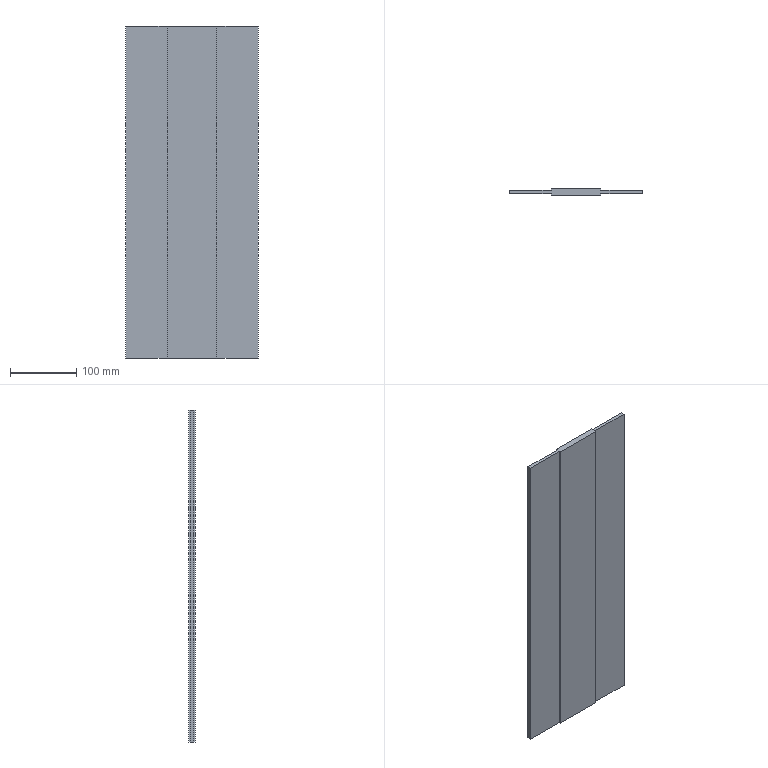Part | SolidWorks | features Extrusion 1, ICE 1 | 1 solid | 14 faces | box 200 x 10 x 500 mm | volume 687500 mm3 | plane 14
STEP:
#1=CARTESIAN_POINT('',(100.,2.5,0.));
#2=VERTEX_POINT('',#1);
#3=CARTESIAN_POINT('',(37.5,2.5,0.));
#4=VERTEX_POINT('',#3);
#5=CARTESIAN_POINT('',(-100.,2.5,0.));
#6=DIRECTION('',(-1.,0.,0.));
#7=VECTOR('',#6,1000.);
#8=LINE('',#5,#7);
#9=EDGE_CURVE('',#2,#4,#8,.T.);
#10=ORIENTED_EDGE('',*,*,#9,.T.);
#11=CARTESIAN_POINT('',(37.5,2.5,500.));
#12=VERTEX_POINT('',#11);
#13=CARTESIAN_POINT('',(37.5,2.5,500.));
#14=DIRECTION('',(0.,0.,1.));
#15=VECTOR('',#14,1000.);
#16=LINE('',#13,#15);
#17=EDGE_CURVE('',#4,#12,#16,.T.);
#18=ORIENTED_EDGE('',*,*,#17,.T.);
#19=CARTESIAN_POINT('',(100.,2.5,500.));
#20=VERTEX_POINT('',#19);
#21=CARTESIAN_POINT('',(-100.,2.5,500.));
#22=DIRECTION('',(-1.,0.,0.));
#23=VECTOR('',#22,1000.);
#24=LINE('',#21,#23);
#25=EDGE_CURVE('',#20,#12,#24,.T.);
#26=ORIENTED_EDGE('',*,*,#25,.F.);
#27=CARTESIAN_POINT('',(100.,2.5,500.));
#28=DIRECTION('',(0.,0.,-1.));
#29=VECTOR('',#28,1000.);
#30=LINE('',#27,#29);
#31=EDGE_CURVE('',#20,#2,#30,.T.);
#32=ORIENTED_EDGE('',*,*,#31,.T.);
#33=EDGE_LOOP('',(#10,#18,#26,#32));
#34=FACE_OUTER_BOUND('',#33,.T.);
#35=CARTESIAN_POINT('',(-100.,2.5,500.));
#36=DIRECTION('',(0.,-1.,0.));
#37=DIRECTION('',(0.,0.,-1.));
#38=AXIS2_PLACEMENT_3D('',#35,#36,#37);
#39=PLANE('',#38);
#40=ADVANCED_FACE('',(#34),#39,.F.);
#41=CARTESIAN_POINT('',(37.5,-2.5,500.));
#42=VERTEX_POINT('',#41);
#43=CARTESIAN_POINT('',(100.,-2.5,500.));
#44=VERTEX_POINT('',#43);
#45=CARTESIAN_POINT('',(-100.,-2.5,500.));
#46=DIRECTION('',(1.,0.,0.));
#47=VECTOR('',#46,1000.);
#48=LINE('',#45,#47);
#49=EDGE_CURVE('',#42,#44,#48,.T.);
#50=ORIENTED_EDGE('',*,*,#49,.F.);
#51=CARTESIAN_POINT('',(37.5,-2.5,0.));
#52=VERTEX_POINT('',#51);
#53=CARTESIAN_POINT('',(37.5,-2.5,500.));
#54=DIRECTION('',(0.,0.,-1.));
#55=VECTOR('',#54,1000.);
#56=LINE('',#53,#55);
#57=EDGE_CURVE('',#42,#52,#56,.T.);
#58=ORIENTED_EDGE('',*,*,#57,.T.);
#59=CARTESIAN_POINT('',(100.,-2.5,0.));
#60=VERTEX_POINT('',#59);
#61=CARTESIAN_POINT('',(-100.,-2.5,0.));
#62=DIRECTION('',(1.,0.,0.));
#63=VECTOR('',#62,1000.);
#64=LINE('',#61,#63);
#65=EDGE_CURVE('',#52,#60,#64,.T.);
#66=ORIENTED_EDGE('',*,*,#65,.T.);
#67=CARTESIAN_POINT('',(100.,-2.5,500.));
#68=DIRECTION('',(0.,0.,-1.));
#69=VECTOR('',#68,1000.);
#70=LINE('',#67,#69);
#71=EDGE_CURVE('',#44,#60,#70,.T.);
#72=ORIENTED_EDGE('',*,*,#71,.F.);
#73=EDGE_LOOP('',(#50,#58,#66,#72));
#74=FACE_OUTER_BOUND('',#73,.T.);
#75=CARTESIAN_POINT('',(-100.,-2.5,500.));
#76=DIRECTION('',(0.,1.,0.));
#77=DIRECTION('',(0.,0.,1.));
#78=AXIS2_PLACEMENT_3D('',#75,#76,#77);
#79=PLANE('',#78);
#80=ADVANCED_FACE('',(#74),#79,.F.);
#81=CARTESIAN_POINT('',(100.,2.5,0.));
#82=DIRECTION('',(0.,1.,0.));
#83=VECTOR('',#82,1000.);
#84=LINE('',#81,#83);
#85=EDGE_CURVE('',#60,#2,#84,.T.);
#86=ORIENTED_EDGE('',*,*,#85,.T.);
#87=ORIENTED_EDGE('',*,*,#31,.F.);
#88=CARTESIAN_POINT('',(100.,2.5,500.));
#89=DIRECTION('',(0.,1.,0.));
#90=VECTOR('',#89,1000.);
#91=LINE('',#88,#90);
#92=EDGE_CURVE('',#44,#20,#91,.T.);
#93=ORIENTED_EDGE('',*,*,#92,.F.);
#94=ORIENTED_EDGE('',*,*,#71,.T.);
#95=EDGE_LOOP('',(#86,#87,#93,#94));
#96=FACE_OUTER_BOUND('',#95,.T.);
#97=CARTESIAN_POINT('',(100.,2.5,500.));
#98=DIRECTION('',(-1.,0.,0.));
#99=DIRECTION('',(0.,0.,1.));
#100=AXIS2_PLACEMENT_3D('',#97,#98,#99);
#101=PLANE('',#100);
#102=ADVANCED_FACE('',(#96),#101,.F.);
#103=CARTESIAN_POINT('',(-37.5,2.5,500.));
#104=VERTEX_POINT('',#103);
#105=CARTESIAN_POINT('',(-100.,2.5,500.));
#106=VERTEX_POINT('',#105);
#107=CARTESIAN_POINT('',(-100.,2.5,500.));
#108=DIRECTION('',(-1.,0.,0.));
#109=VECTOR('',#108,1000.);
#110=LINE('',#107,#109);
#111=EDGE_CURVE('',#104,#106,#110,.T.);
#112=ORIENTED_EDGE('',*,*,#111,.F.);
#113=CARTESIAN_POINT('',(-37.5,2.5,0.));
#114=VERTEX_POINT('',#113);
#115=CARTESIAN_POINT('',(-37.5,2.5,500.));
#116=DIRECTION('',(0.,0.,-1.));
#117=VECTOR('',#116,1000.);
#118=LINE('',#115,#117);
#119=EDGE_CURVE('',#104,#114,#118,.T.);
#120=ORIENTED_EDGE('',*,*,#119,.T.);
#121=CARTESIAN_POINT('',(-100.,2.5,0.));
#122=VERTEX_POINT('',#121);
#123=CARTESIAN_POINT('',(-100.,2.5,0.));
#124=DIRECTION('',(-1.,0.,0.));
#125=VECTOR('',#124,1000.);
#126=LINE('',#123,#125);
#127=EDGE_CURVE('',#114,#122,#126,.T.);
#128=ORIENTED_EDGE('',*,*,#127,.T.);
#129=CARTESIAN_POINT('',(-100.,2.5,500.));
#130=DIRECTION('',(0.,0.,-1.));
#131=VECTOR('',#130,1000.);
#132=LINE('',#129,#131);
#133=EDGE_CURVE('',#106,#122,#132,.T.);
#134=ORIENTED_EDGE('',*,*,#133,.F.);
#135=EDGE_LOOP('',(#112,#120,#128,#134));
#136=FACE_OUTER_BOUND('',#135,.T.);
#137=CARTESIAN_POINT('',(-100.,2.5,500.));
#138=DIRECTION('',(0.,-1.,0.));
#139=DIRECTION('',(0.,0.,-1.));
#140=AXIS2_PLACEMENT_3D('',#137,#138,#139);
#141=PLANE('',#140);
#142=ADVANCED_FACE('',(#136),#141,.F.);
#143=CARTESIAN_POINT('',(-100.,-2.5,0.));
#144=VERTEX_POINT('',#143);
#145=CARTESIAN_POINT('',(-100.,2.5,0.));
#146=DIRECTION('',(0.,-1.,0.));
#147=VECTOR('',#146,1000.);
#148=LINE('',#145,#147);
#149=EDGE_CURVE('',#122,#144,#148,.T.);
#150=ORIENTED_EDGE('',*,*,#149,.T.);
#151=CARTESIAN_POINT('',(-100.,-2.5,500.));
#152=VERTEX_POINT('',#151);
#153=CARTESIAN_POINT('',(-100.,-2.5,500.));
#154=DIRECTION('',(0.,0.,-1.));
#155=VECTOR('',#154,1000.);
#156=LINE('',#153,#155);
#157=EDGE_CURVE('',#152,#144,#156,.T.);
#158=ORIENTED_EDGE('',*,*,#157,.F.);
#159=CARTESIAN_POINT('',(-100.,2.5,500.));
#160=DIRECTION('',(0.,-1.,0.));
#161=VECTOR('',#160,1000.);
#162=LINE('',#159,#161);
#163=EDGE_CURVE('',#106,#152,#162,.T.);
#164=ORIENTED_EDGE('',*,*,#163,.F.);
#165=ORIENTED_EDGE('',*,*,#133,.T.);
#166=EDGE_LOOP('',(#150,#158,#164,#165));
#167=FACE_OUTER_BOUND('',#166,.T.);
#168=CARTESIAN_POINT('',(-100.,2.5,500.));
#169=DIRECTION('',(1.,0.,0.));
#170=DIRECTION('',(0.,0.,-1.));
#171=AXIS2_PLACEMENT_3D('',#168,#169,#170);
#172=PLANE('',#171);
#173=ADVANCED_FACE('',(#167),#172,.F.);
#174=CARTESIAN_POINT('',(-37.5,-2.5,0.));
#175=VERTEX_POINT('',#174);
#176=CARTESIAN_POINT('',(-100.,-2.5,0.));
#177=DIRECTION('',(1.,0.,0.));
#178=VECTOR('',#177,1000.);
#179=LINE('',#176,#178);
#180=EDGE_CURVE('',#144,#175,#179,.T.);
#181=ORIENTED_EDGE('',*,*,#180,.T.);
#182=CARTESIAN_POINT('',(-37.5,-2.5,500.));
#183=VERTEX_POINT('',#182);
#184=CARTESIAN_POINT('',(-37.5,-2.5,500.));
#185=DIRECTION('',(0.,0.,1.));
#186=VECTOR('',#185,1000.);
#187=LINE('',#184,#186);
#188=EDGE_CURVE('',#175,#183,#187,.T.);
#189=ORIENTED_EDGE('',*,*,#188,.T.);
#190=CARTESIAN_POINT('',(-100.,-2.5,500.));
#191=DIRECTION('',(1.,0.,0.));
#192=VECTOR('',#191,1000.);
#193=LINE('',#190,#192);
#194=EDGE_CURVE('',#152,#183,#193,.T.);
#195=ORIENTED_EDGE('',*,*,#194,.F.);
#196=ORIENTED_EDGE('',*,*,#157,.T.);
#197=EDGE_LOOP('',(#181,#189,#195,#196));
#198=FACE_OUTER_BOUND('',#197,.T.);
#199=CARTESIAN_POINT('',(-100.,-2.5,500.));
#200=DIRECTION('',(0.,1.,0.));
#201=DIRECTION('',(0.,0.,1.));
#202=AXIS2_PLACEMENT_3D('',#199,#200,#201);
#203=PLANE('',#202);
#204=ADVANCED_FACE('',(#198),#203,.F.);
#205=ORIENTED_EDGE('',*,*,#194,.T.);
#206=CARTESIAN_POINT('',(-37.5,-5.,500.));
#207=VERTEX_POINT('',#206);
#208=CARTESIAN_POINT('',(-37.5,5.,500.));
#209=DIRECTION('',(0.,-1.,0.));
#210=VECTOR('',#209,1000.);
#211=LINE('',#208,#210);
#212=EDGE_CURVE('',#183,#207,#211,.T.);
#213=ORIENTED_EDGE('',*,*,#212,.T.);
#214=CARTESIAN_POINT('',(37.5,-5.,500.));
#215=VERTEX_POINT('',#214);
#216=CARTESIAN_POINT('',(-37.5,-5.,500.));
#217=DIRECTION('',(1.,0.,0.));
#218=VECTOR('',#217,1000.);
#219=LINE('',#216,#218);
#220=EDGE_CURVE('',#207,#215,#219,.T.);
#221=ORIENTED_EDGE('',*,*,#220,.T.);
#222=CARTESIAN_POINT('',(37.5,5.,500.));
#223=DIRECTION('',(0.,1.,0.));
#224=VECTOR('',#223,1000.);
#225=LINE('',#222,#224);
#226=EDGE_CURVE('',#215,#42,#225,.T.);
#227=ORIENTED_EDGE('',*,*,#226,.T.);
#228=ORIENTED_EDGE('',*,*,#49,.T.);
#229=ORIENTED_EDGE('',*,*,#92,.T.);
#230=ORIENTED_EDGE('',*,*,#25,.T.);
#231=CARTESIAN_POINT('',(37.5,5.,500.));
#232=VERTEX_POINT('',#231);
#233=CARTESIAN_POINT('',(37.5,5.,500.));
#234=DIRECTION('',(0.,1.,0.));
#235=VECTOR('',#234,1000.);
#236=LINE('',#233,#235);
#237=EDGE_CURVE('',#12,#232,#236,.T.);
#238=ORIENTED_EDGE('',*,*,#237,.T.);
#239=CARTESIAN_POINT('',(-37.5,5.,500.));
#240=VERTEX_POINT('',#239);
#241=CARTESIAN_POINT('',(-37.5,5.,500.));
#242=DIRECTION('',(-1.,0.,0.));
#243=VECTOR('',#242,1000.);
#244=LINE('',#241,#243);
#245=EDGE_CURVE('',#232,#240,#244,.T.);
#246=ORIENTED_EDGE('',*,*,#245,.T.);
#247=CARTESIAN_POINT('',(-37.5,5.,500.));
#248=DIRECTION('',(0.,-1.,0.));
#249=VECTOR('',#248,1000.);
#250=LINE('',#247,#249);
#251=EDGE_CURVE('',#240,#104,#250,.T.);
#252=ORIENTED_EDGE('',*,*,#251,.T.);
#253=ORIENTED_EDGE('',*,*,#111,.T.);
#254=ORIENTED_EDGE('',*,*,#163,.T.);
#255=EDGE_LOOP('',(#205,#213,#221,#227,#228,#229,#230,#238,#246,#252,#253,#254));
#256=FACE_OUTER_BOUND('',#255,.T.);
#257=CARTESIAN_POINT('',(0.,0.,500.));
#258=DIRECTION('',(0.,0.,1.));
#259=DIRECTION('',(1.,0.,0.));
#260=AXIS2_PLACEMENT_3D('',#257,#258,#259);
#261=PLANE('',#260);
#262=ADVANCED_FACE('',(#256),#261,.T.);
#263=ORIENTED_EDGE('',*,*,#127,.F.);
#264=CARTESIAN_POINT('',(-37.5,5.,0.));
#265=VERTEX_POINT('',#264);
#266=CARTESIAN_POINT('',(-37.5,5.,0.));
#267=DIRECTION('',(0.,-1.,0.));
#268=VECTOR('',#267,1000.);
#269=LINE('',#266,#268);
#270=EDGE_CURVE('',#265,#114,#269,.T.);
#271=ORIENTED_EDGE('',*,*,#270,.F.);
#272=CARTESIAN_POINT('',(37.5,5.,0.));
#273=VERTEX_POINT('',#272);
#274=CARTESIAN_POINT('',(-37.5,5.,0.));
#275=DIRECTION('',(-1.,0.,0.));
#276=VECTOR('',#275,1000.);
#277=LINE('',#274,#276);
#278=EDGE_CURVE('',#273,#265,#277,.T.);
#279=ORIENTED_EDGE('',*,*,#278,.F.);
#280=CARTESIAN_POINT('',(37.5,5.,0.));
#281=DIRECTION('',(0.,1.,0.));
#282=VECTOR('',#281,1000.);
#283=LINE('',#280,#282);
#284=EDGE_CURVE('',#4,#273,#283,.T.);
#285=ORIENTED_EDGE('',*,*,#284,.F.);
#286=ORIENTED_EDGE('',*,*,#9,.F.);
#287=ORIENTED_EDGE('',*,*,#85,.F.);
#288=ORIENTED_EDGE('',*,*,#65,.F.);
#289=CARTESIAN_POINT('',(37.5,-5.,0.));
#290=VERTEX_POINT('',#289);
#291=CARTESIAN_POINT('',(37.5,5.,0.));
#292=DIRECTION('',(0.,1.,0.));
#293=VECTOR('',#292,1000.);
#294=LINE('',#291,#293);
#295=EDGE_CURVE('',#290,#52,#294,.T.);
#296=ORIENTED_EDGE('',*,*,#295,.F.);
#297=CARTESIAN_POINT('',(-37.5,-5.,0.));
#298=VERTEX_POINT('',#297);
#299=CARTESIAN_POINT('',(-37.5,-5.,0.));
#300=DIRECTION('',(1.,0.,0.));
#301=VECTOR('',#300,1000.);
#302=LINE('',#299,#301);
#303=EDGE_CURVE('',#298,#290,#302,.T.);
#304=ORIENTED_EDGE('',*,*,#303,.F.);
#305=CARTESIAN_POINT('',(-37.5,5.,0.));
#306=DIRECTION('',(0.,-1.,0.));
#307=VECTOR('',#306,1000.);
#308=LINE('',#305,#307);
#309=EDGE_CURVE('',#175,#298,#308,.T.);
#310=ORIENTED_EDGE('',*,*,#309,.F.);
#311=ORIENTED_EDGE('',*,*,#180,.F.);
#312=ORIENTED_EDGE('',*,*,#149,.F.);
#313=EDGE_LOOP('',(#263,#271,#279,#285,#286,#287,#288,#296,#304,#310,#311,#312));
#314=FACE_OUTER_BOUND('',#313,.T.);
#315=CARTESIAN_POINT('',(0.,0.,0.));
#316=DIRECTION('',(0.,0.,1.));
#317=DIRECTION('',(1.,0.,0.));
#318=AXIS2_PLACEMENT_3D('',#315,#316,#317);
#319=PLANE('',#318);
#320=ADVANCED_FACE('',(#314),#319,.F.);
#321=ORIENTED_EDGE('',*,*,#220,.F.);
#322=CARTESIAN_POINT('',(-37.5,-5.,0.));
#323=DIRECTION('',(0.,0.,1.));
#324=VECTOR('',#323,1000.);
#325=LINE('',#322,#324);
#326=EDGE_CURVE('',#298,#207,#325,.T.);
#327=ORIENTED_EDGE('',*,*,#326,.F.);
#328=ORIENTED_EDGE('',*,*,#303,.T.);
#329=CARTESIAN_POINT('',(37.5,-5.,0.));
#330=DIRECTION('',(0.,0.,1.));
#331=VECTOR('',#330,1000.);
#332=LINE('',#329,#331);
#333=EDGE_CURVE('',#290,#215,#332,.T.);
#334=ORIENTED_EDGE('',*,*,#333,.T.);
#335=EDGE_LOOP('',(#321,#327,#328,#334));
#336=FACE_OUTER_BOUND('',#335,.T.);
#337=CARTESIAN_POINT('',(-37.5,-5.,0.));
#338=DIRECTION('',(0.,-1.,0.));
#339=DIRECTION('',(0.,0.,-1.));
#340=AXIS2_PLACEMENT_3D('',#337,#338,#339);
#341=PLANE('',#340);
#342=ADVANCED_FACE('',(#336),#341,.T.);
#343=ORIENTED_EDGE('',*,*,#188,.F.);
#344=ORIENTED_EDGE('',*,*,#309,.T.);
#345=ORIENTED_EDGE('',*,*,#326,.T.);
#346=ORIENTED_EDGE('',*,*,#212,.F.);
#347=EDGE_LOOP('',(#343,#344,#345,#346));
#348=FACE_OUTER_BOUND('',#347,.T.);
#349=CARTESIAN_POINT('',(-37.5,5.,0.));
#350=DIRECTION('',(-1.,0.,0.));
#351=DIRECTION('',(0.,0.,1.));
#352=AXIS2_PLACEMENT_3D('',#349,#350,#351);
#353=PLANE('',#352);
#354=ADVANCED_FACE('',(#348),#353,.T.);
#355=ORIENTED_EDGE('',*,*,#57,.F.);
#356=ORIENTED_EDGE('',*,*,#226,.F.);
#357=ORIENTED_EDGE('',*,*,#333,.F.);
#358=ORIENTED_EDGE('',*,*,#295,.T.);
#359=EDGE_LOOP('',(#355,#356,#357,#358));
#360=FACE_OUTER_BOUND('',#359,.T.);
#361=CARTESIAN_POINT('',(37.5,5.,0.));
#362=DIRECTION('',(1.,0.,0.));
#363=DIRECTION('',(0.,0.,-1.));
#364=AXIS2_PLACEMENT_3D('',#361,#362,#363);
#365=PLANE('',#364);
#366=ADVANCED_FACE('',(#360),#365,.T.);
#367=ORIENTED_EDGE('',*,*,#17,.F.);
#368=ORIENTED_EDGE('',*,*,#284,.T.);
#369=CARTESIAN_POINT('',(37.5,5.,0.));
#370=DIRECTION('',(0.,0.,1.));
#371=VECTOR('',#370,1000.);
#372=LINE('',#369,#371);
#373=EDGE_CURVE('',#273,#232,#372,.T.);
#374=ORIENTED_EDGE('',*,*,#373,.T.);
#375=ORIENTED_EDGE('',*,*,#237,.F.);
#376=EDGE_LOOP('',(#367,#368,#374,#375));
#377=FACE_OUTER_BOUND('',#376,.T.);
#378=CARTESIAN_POINT('',(37.5,5.,0.));
#379=DIRECTION('',(1.,0.,0.));
#380=DIRECTION('',(0.,0.,-1.));
#381=AXIS2_PLACEMENT_3D('',#378,#379,#380);
#382=PLANE('',#381);
#383=ADVANCED_FACE('',(#377),#382,.T.);
#384=ORIENTED_EDGE('',*,*,#119,.F.);
#385=ORIENTED_EDGE('',*,*,#251,.F.);
#386=CARTESIAN_POINT('',(-37.5,5.,0.));
#387=DIRECTION('',(0.,0.,1.));
#388=VECTOR('',#387,1000.);
#389=LINE('',#386,#388);
#390=EDGE_CURVE('',#265,#240,#389,.T.);
#391=ORIENTED_EDGE('',*,*,#390,.F.);
#392=ORIENTED_EDGE('',*,*,#270,.T.);
#393=EDGE_LOOP('',(#384,#385,#391,#392));
#394=FACE_OUTER_BOUND('',#393,.T.);
#395=CARTESIAN_POINT('',(-37.5,5.,0.));
#396=DIRECTION('',(-1.,0.,0.));
#397=DIRECTION('',(0.,0.,1.));
#398=AXIS2_PLACEMENT_3D('',#395,#396,#397);
#399=PLANE('',#398);
#400=ADVANCED_FACE('',(#394),#399,.T.);
#401=ORIENTED_EDGE('',*,*,#245,.F.);
#402=ORIENTED_EDGE('',*,*,#373,.F.);
#403=ORIENTED_EDGE('',*,*,#278,.T.);
#404=ORIENTED_EDGE('',*,*,#390,.T.);
#405=EDGE_LOOP('',(#401,#402,#403,#404));
#406=FACE_OUTER_BOUND('',#405,.T.);
#407=CARTESIAN_POINT('',(-37.5,5.,0.));
#408=DIRECTION('',(0.,1.,0.));
#409=DIRECTION('',(0.,0.,1.));
#410=AXIS2_PLACEMENT_3D('',#407,#408,#409);
#411=PLANE('',#410);
#412=ADVANCED_FACE('',(#406),#411,.T.);
#413=CLOSED_SHELL('',(#40,#80,#102,#142,#173,#204,#262,#320,#342,#354,#366,#383,#400,#412));
#414=MANIFOLD_SOLID_BREP('',#413);
#415=CARTESIAN_POINT('',(0.,0.,0.));
#416=DIRECTION('',(0.,0.,1.));
#417=DIRECTION('',(1.,0.,0.));
#418=AXIS2_PLACEMENT_3D('',#415,#416,#417);
#419=(LENGTH_UNIT()NAMED_UNIT(*)SI_UNIT(.MILLI.,.METRE.));
#420=UNCERTAINTY_MEASURE_WITH_UNIT(LENGTH_MEASURE(0.00001),#419,'','');
#421=(NAMED_UNIT(*)PLANE_ANGLE_UNIT()SI_UNIT($,.RADIAN.));
#422=(NAMED_UNIT(*)SI_UNIT($,.STERADIAN.)SOLID_ANGLE_UNIT());
#423=(GEOMETRIC_REPRESENTATION_CONTEXT(3)GLOBAL_UNCERTAINTY_ASSIGNED_CONTEXT((#420))GLOBAL_UNIT_ASSIGNED_CONTEXT((#419,#421,#422))REPRESENTATION_CONTEXT('',''));
#424=ADVANCED_BREP_SHAPE_REPRESENTATION('',(#414,#418),#423);